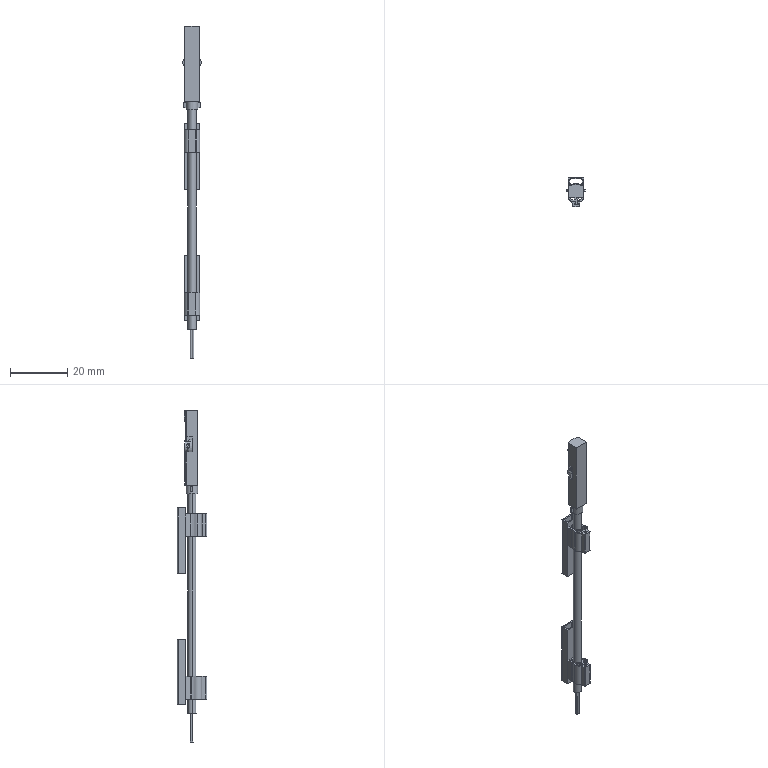Part | SolidWorks | 3 solids | 271 faces | box 6.45 x 10.3 x 116.3 mm | volume 1707 mm3 | plane 150 | cylinder 119 | cone 2 | commonest cylinder face diameters 0.4 x29 0.6 x24 0.45 x8 6.82 x8 0.2 x6 2 x6